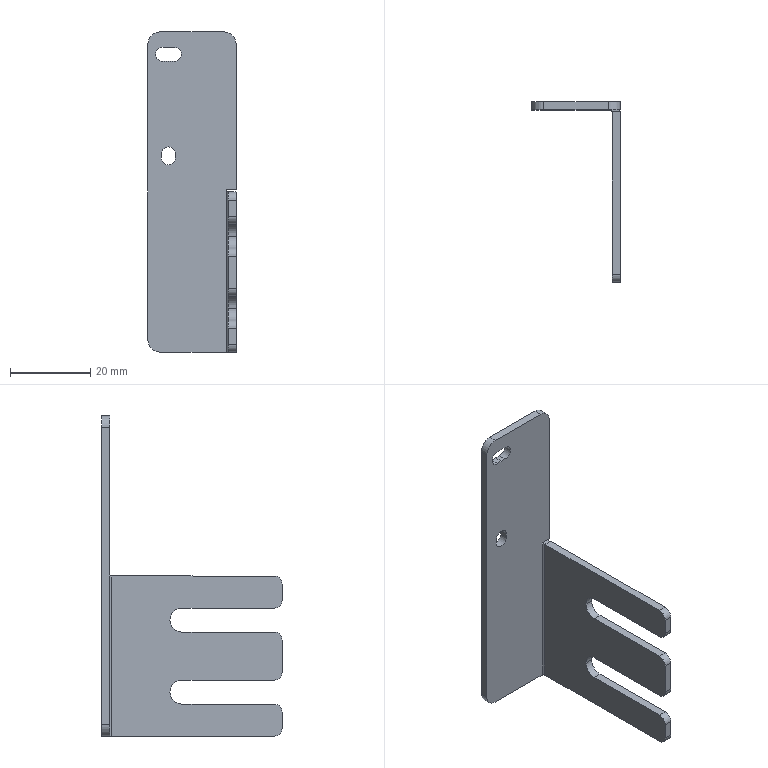Part | SolidWorks | features ICE 4, Fillet 2, ExtruThin 1, FlatPattern 1, FlattenBends 1, ProcessBends 1, SheetMetal 1 | 1 solid | 47 faces | box 22 x 45 x 80 mm | volume 6161 mm3 | cylinder 24 | plane 23 | commonest cylinder face diameters 6 x7 4 x6 3.5 x5 47.3 x2 54.3 x2 1 x1
STEP:
#1=CARTESIAN_POINT('',(-2.,-17.,29.));
#2=VERTEX_POINT('',#1);
#3=CARTESIAN_POINT('',(-2.,-20.,32.));
#4=VERTEX_POINT('',#3);
#5=CARTESIAN_POINT('',(-2.,-20.,29.));
#6=DIRECTION('',(1.,0.,0.));
#7=DIRECTION('',(0.,1.,0.));
#8=AXIS2_PLACEMENT_3D('',#5,#6,#7);
#9=CIRCLE('',#8,3.);
#10=EDGE_CURVE('',#2,#4,#9,.T.);
#11=ORIENTED_EDGE('',*,*,#10,.F.);
#12=CARTESIAN_POINT('',(0.,-17.,29.));
#13=VERTEX_POINT('',#12);
#14=CARTESIAN_POINT('',(-116.726,-17.,29.));
#15=DIRECTION('',(1.,0.,0.));
#16=VECTOR('',#15,1000.);
#17=LINE('',#14,#16);
#18=EDGE_CURVE('',#2,#13,#17,.T.);
#19=ORIENTED_EDGE('',*,*,#18,.T.);
#20=CARTESIAN_POINT('',(0.,-20.,32.));
#21=VERTEX_POINT('',#20);
#22=CARTESIAN_POINT('',(0.,-20.,29.));
#23=DIRECTION('',(1.,0.,0.));
#24=DIRECTION('',(0.,1.,0.));
#25=AXIS2_PLACEMENT_3D('',#22,#23,#24);
#26=CIRCLE('',#25,3.);
#27=EDGE_CURVE('',#13,#21,#26,.T.);
#28=ORIENTED_EDGE('',*,*,#27,.T.);
#29=CARTESIAN_POINT('',(-116.726,-20.,32.));
#30=DIRECTION('',(1.,0.,0.));
#31=VECTOR('',#30,1000.);
#32=LINE('',#29,#31);
#33=EDGE_CURVE('',#4,#21,#32,.T.);
#34=ORIENTED_EDGE('',*,*,#33,.F.);
#35=EDGE_LOOP('',(#11,#19,#28,#34));
#36=FACE_OUTER_BOUND('',#35,.T.);
#37=CARTESIAN_POINT('',(-116.726,-20.,29.));
#38=DIRECTION('',(1.,0.,0.));
#39=DIRECTION('',(0.,1.,0.));
#40=AXIS2_PLACEMENT_3D('',#37,#38,#39);
#41=CYLINDRICAL_SURFACE('',#40,3.);
#42=ADVANCED_FACE('',(#36),#41,.F.);
#43=CARTESIAN_POINT('',(-2.,-17.,11.));
#44=VERTEX_POINT('',#43);
#45=CARTESIAN_POINT('',(-2.,-20.,14.));
#46=VERTEX_POINT('',#45);
#47=CARTESIAN_POINT('',(-2.,-20.,11.));
#48=DIRECTION('',(1.,0.,0.));
#49=DIRECTION('',(0.,1.,0.));
#50=AXIS2_PLACEMENT_3D('',#47,#48,#49);
#51=CIRCLE('',#50,3.);
#52=EDGE_CURVE('',#44,#46,#51,.T.);
#53=ORIENTED_EDGE('',*,*,#52,.F.);
#54=CARTESIAN_POINT('',(0.,-17.,11.));
#55=VERTEX_POINT('',#54);
#56=CARTESIAN_POINT('',(-116.726,-17.,11.));
#57=DIRECTION('',(1.,0.,0.));
#58=VECTOR('',#57,1000.);
#59=LINE('',#56,#58);
#60=EDGE_CURVE('',#44,#55,#59,.T.);
#61=ORIENTED_EDGE('',*,*,#60,.T.);
#62=CARTESIAN_POINT('',(0.,-20.,14.));
#63=VERTEX_POINT('',#62);
#64=CARTESIAN_POINT('',(0.,-20.,11.));
#65=DIRECTION('',(1.,0.,0.));
#66=DIRECTION('',(0.,-1.,0.));
#67=AXIS2_PLACEMENT_3D('',#64,#65,#66);
#68=CIRCLE('',#67,3.);
#69=EDGE_CURVE('',#55,#63,#68,.T.);
#70=ORIENTED_EDGE('',*,*,#69,.T.);
#71=CARTESIAN_POINT('',(-116.726,-20.,14.));
#72=DIRECTION('',(1.,0.,0.));
#73=VECTOR('',#72,1000.);
#74=LINE('',#71,#73);
#75=EDGE_CURVE('',#46,#63,#74,.T.);
#76=ORIENTED_EDGE('',*,*,#75,.F.);
#77=EDGE_LOOP('',(#53,#61,#70,#76));
#78=FACE_OUTER_BOUND('',#77,.T.);
#79=CARTESIAN_POINT('',(-116.726,-20.,11.));
#80=DIRECTION('',(1.,0.,0.));
#81=DIRECTION('',(0.,1.,0.));
#82=AXIS2_PLACEMENT_3D('',#79,#80,#81);
#83=CYLINDRICAL_SURFACE('',#82,3.);
#84=ADVANCED_FACE('',(#78),#83,.F.);
#85=CARTESIAN_POINT('',(-16.893,-2.,51.25));
#86=VERTEX_POINT('',#85);
#87=CARTESIAN_POINT('',(-15.143,-2.,49.5));
#88=VERTEX_POINT('',#87);
#89=CARTESIAN_POINT('',(-16.893,-2.,49.5));
#90=DIRECTION('',(0.,1.,0.));
#91=DIRECTION('',(0.,0.,1.));
#92=AXIS2_PLACEMENT_3D('',#89,#90,#91);
#93=CIRCLE('',#92,1.75);
#94=EDGE_CURVE('',#86,#88,#93,.T.);
#95=ORIENTED_EDGE('',*,*,#94,.F.);
#96=CARTESIAN_POINT('',(-16.893,0.,51.25));
#97=VERTEX_POINT('',#96);
#98=CARTESIAN_POINT('',(-16.893,-10.,51.25));
#99=DIRECTION('',(0.,1.,0.));
#100=VECTOR('',#99,1000.);
#101=LINE('',#98,#100);
#102=EDGE_CURVE('',#86,#97,#101,.T.);
#103=ORIENTED_EDGE('',*,*,#102,.T.);
#104=CARTESIAN_POINT('',(-15.143,0.,49.5));
#105=VERTEX_POINT('',#104);
#106=CARTESIAN_POINT('',(-16.893,0.,49.5));
#107=DIRECTION('',(0.,1.,0.));
#108=DIRECTION('',(0.,0.,1.));
#109=AXIS2_PLACEMENT_3D('',#106,#107,#108);
#110=CIRCLE('',#109,1.75);
#111=EDGE_CURVE('',#97,#105,#110,.T.);
#112=ORIENTED_EDGE('',*,*,#111,.T.);
#113=CARTESIAN_POINT('',(-15.143,-10.,49.5));
#114=DIRECTION('',(0.,1.,0.));
#115=VECTOR('',#114,1000.);
#116=LINE('',#113,#115);
#117=EDGE_CURVE('',#88,#105,#116,.T.);
#118=ORIENTED_EDGE('',*,*,#117,.F.);
#119=EDGE_LOOP('',(#95,#103,#112,#118));
#120=FACE_OUTER_BOUND('',#119,.T.);
#121=CARTESIAN_POINT('',(-16.893,-10.,49.5));
#122=DIRECTION('',(0.,1.,0.));
#123=DIRECTION('',(0.,0.,1.));
#124=AXIS2_PLACEMENT_3D('',#121,#122,#123);
#125=CYLINDRICAL_SURFACE('',#124,1.75);
#126=ADVANCED_FACE('',(#120),#125,.F.);
#127=CARTESIAN_POINT('',(-16.893,-2.,72.65));
#128=VERTEX_POINT('',#127);
#129=CARTESIAN_POINT('',(-18.289,-2.,72.609));
#130=VERTEX_POINT('',#129);
#131=CARTESIAN_POINT('',(-16.893,-2.,49.));
#132=DIRECTION('',(0.,-1.,0.));
#133=DIRECTION('',(0.,0.,1.));
#134=AXIS2_PLACEMENT_3D('',#131,#132,#133);
#135=CIRCLE('',#134,23.65);
#136=EDGE_CURVE('',#128,#130,#135,.T.);
#137=ORIENTED_EDGE('',*,*,#136,.F.);
#138=CARTESIAN_POINT('',(-16.893,0.,72.65));
#139=VERTEX_POINT('',#138);
#140=CARTESIAN_POINT('',(-16.893,-10.,72.65));
#141=DIRECTION('',(0.,1.,0.));
#142=VECTOR('',#141,1000.);
#143=LINE('',#140,#142);
#144=EDGE_CURVE('',#128,#139,#143,.T.);
#145=ORIENTED_EDGE('',*,*,#144,.T.);
#146=CARTESIAN_POINT('',(-18.289,0.,72.609));
#147=VERTEX_POINT('',#146);
#148=CARTESIAN_POINT('',(-16.893,0.,49.));
#149=DIRECTION('',(0.,-1.,0.));
#150=DIRECTION('',(0.,0.,1.));
#151=AXIS2_PLACEMENT_3D('',#148,#149,#150);
#152=CIRCLE('',#151,23.65);
#153=EDGE_CURVE('',#139,#147,#152,.T.);
#154=ORIENTED_EDGE('',*,*,#153,.T.);
#155=CARTESIAN_POINT('',(-18.289,-10.,72.609));
#156=DIRECTION('',(0.,1.,0.));
#157=VECTOR('',#156,1000.);
#158=LINE('',#155,#157);
#159=EDGE_CURVE('',#130,#147,#158,.T.);
#160=ORIENTED_EDGE('',*,*,#159,.F.);
#161=EDGE_LOOP('',(#137,#145,#154,#160));
#162=FACE_OUTER_BOUND('',#161,.T.);
#163=CARTESIAN_POINT('',(-16.893,-10.,49.));
#164=DIRECTION('',(0.,1.,0.));
#165=DIRECTION('',(0.,0.,1.));
#166=AXIS2_PLACEMENT_3D('',#163,#164,#165);
#167=CYLINDRICAL_SURFACE('',#166,23.65);
#168=ADVANCED_FACE('',(#162),#167,.T.);
#169=CARTESIAN_POINT('',(-16.893,-2.,76.15));
#170=VERTEX_POINT('',#169);
#171=CARTESIAN_POINT('',(-15.289,-2.,76.103));
#172=VERTEX_POINT('',#171);
#173=CARTESIAN_POINT('',(-16.893,-2.,49.));
#174=DIRECTION('',(0.,1.,0.));
#175=DIRECTION('',(0.,0.,1.));
#176=AXIS2_PLACEMENT_3D('',#173,#174,#175);
#177=CIRCLE('',#176,27.15);
#178=EDGE_CURVE('',#170,#172,#177,.T.);
#179=ORIENTED_EDGE('',*,*,#178,.F.);
#180=CARTESIAN_POINT('',(-16.893,0.,76.15));
#181=VERTEX_POINT('',#180);
#182=CARTESIAN_POINT('',(-16.893,-10.,76.15));
#183=DIRECTION('',(0.,1.,0.));
#184=VECTOR('',#183,1000.);
#185=LINE('',#182,#184);
#186=EDGE_CURVE('',#170,#181,#185,.T.);
#187=ORIENTED_EDGE('',*,*,#186,.T.);
#188=CARTESIAN_POINT('',(-15.289,0.,76.103));
#189=VERTEX_POINT('',#188);
#190=CARTESIAN_POINT('',(-16.893,0.,49.));
#191=DIRECTION('',(0.,1.,0.));
#192=DIRECTION('',(0.,0.,1.));
#193=AXIS2_PLACEMENT_3D('',#190,#191,#192);
#194=CIRCLE('',#193,27.15);
#195=EDGE_CURVE('',#181,#189,#194,.T.);
#196=ORIENTED_EDGE('',*,*,#195,.T.);
#197=CARTESIAN_POINT('',(-15.289,-10.,76.103));
#198=DIRECTION('',(0.,1.,0.));
#199=VECTOR('',#198,1000.);
#200=LINE('',#197,#199);
#201=EDGE_CURVE('',#172,#189,#200,.T.);
#202=ORIENTED_EDGE('',*,*,#201,.F.);
#203=EDGE_LOOP('',(#179,#187,#196,#202));
#204=FACE_OUTER_BOUND('',#203,.T.);
#205=CARTESIAN_POINT('',(-16.893,-10.,49.));
#206=DIRECTION('',(0.,1.,0.));
#207=DIRECTION('',(0.,0.,1.));
#208=AXIS2_PLACEMENT_3D('',#205,#206,#207);
#209=CYLINDRICAL_SURFACE('',#208,27.15);
#210=ADVANCED_FACE('',(#204),#209,.F.);
#211=ORIENTED_EDGE('',*,*,#186,.F.);
#212=CARTESIAN_POINT('',(-18.496,-2.,76.103));
#213=VERTEX_POINT('',#212);
#214=CARTESIAN_POINT('',(-16.893,-2.,49.));
#215=DIRECTION('',(0.,1.,0.));
#216=DIRECTION('',(0.,0.,1.));
#217=AXIS2_PLACEMENT_3D('',#214,#215,#216);
#218=CIRCLE('',#217,27.15);
#219=EDGE_CURVE('',#213,#170,#218,.T.);
#220=ORIENTED_EDGE('',*,*,#219,.F.);
#221=CARTESIAN_POINT('',(-18.496,0.,76.103));
#222=VERTEX_POINT('',#221);
#223=CARTESIAN_POINT('',(-18.496,-10.,76.103));
#224=DIRECTION('',(0.,1.,0.));
#225=VECTOR('',#224,1000.);
#226=LINE('',#223,#225);
#227=EDGE_CURVE('',#213,#222,#226,.T.);
#228=ORIENTED_EDGE('',*,*,#227,.T.);
#229=CARTESIAN_POINT('',(-16.893,0.,49.));
#230=DIRECTION('',(0.,1.,0.));
#231=DIRECTION('',(0.,0.,1.));
#232=AXIS2_PLACEMENT_3D('',#229,#230,#231);
#233=CIRCLE('',#232,27.15);
#234=EDGE_CURVE('',#222,#181,#233,.T.);
#235=ORIENTED_EDGE('',*,*,#234,.T.);
#236=EDGE_LOOP('',(#211,#220,#228,#235));
#237=FACE_OUTER_BOUND('',#236,.T.);
#238=CARTESIAN_POINT('',(-16.893,-10.,49.));
#239=DIRECTION('',(0.,1.,0.));
#240=DIRECTION('',(0.,0.,1.));
#241=AXIS2_PLACEMENT_3D('',#238,#239,#240);
#242=CYLINDRICAL_SURFACE('',#241,27.15);
#243=ADVANCED_FACE('',(#237),#242,.F.);
#244=ORIENTED_EDGE('',*,*,#201,.T.);
#245=CARTESIAN_POINT('',(-15.496,0.,72.609));
#246=VERTEX_POINT('',#245);
#247=CARTESIAN_POINT('',(-15.393,0.,74.356));
#248=DIRECTION('',(0.,1.,0.));
#249=DIRECTION('',(0.,0.,1.));
#250=AXIS2_PLACEMENT_3D('',#247,#248,#249);
#251=CIRCLE('',#250,1.75);
#252=EDGE_CURVE('',#189,#246,#251,.T.);
#253=ORIENTED_EDGE('',*,*,#252,.T.);
#254=CARTESIAN_POINT('',(-15.496,-2.,72.609));
#255=VERTEX_POINT('',#254);
#256=CARTESIAN_POINT('',(-15.496,-10.,72.609));
#257=DIRECTION('',(0.,1.,0.));
#258=VECTOR('',#257,1000.);
#259=LINE('',#256,#258);
#260=EDGE_CURVE('',#255,#246,#259,.T.);
#261=ORIENTED_EDGE('',*,*,#260,.F.);
#262=CARTESIAN_POINT('',(-15.393,-2.,74.356));
#263=DIRECTION('',(0.,1.,0.));
#264=DIRECTION('',(0.,0.,1.));
#265=AXIS2_PLACEMENT_3D('',#262,#263,#264);
#266=CIRCLE('',#265,1.75);
#267=EDGE_CURVE('',#172,#255,#266,.T.);
#268=ORIENTED_EDGE('',*,*,#267,.F.);
#269=EDGE_LOOP('',(#244,#253,#261,#268));
#270=FACE_OUTER_BOUND('',#269,.T.);
#271=CARTESIAN_POINT('',(-15.393,-10.,74.356));
#272=DIRECTION('',(0.,1.,0.));
#273=DIRECTION('',(0.,0.,1.));
#274=AXIS2_PLACEMENT_3D('',#271,#272,#273);
#275=CYLINDRICAL_SURFACE('',#274,1.75);
#276=ADVANCED_FACE('',(#270),#275,.F.);
#277=ORIENTED_EDGE('',*,*,#144,.F.);
#278=CARTESIAN_POINT('',(-16.893,-2.,49.));
#279=DIRECTION('',(0.,-1.,0.));
#280=DIRECTION('',(0.,0.,1.));
#281=AXIS2_PLACEMENT_3D('',#278,#279,#280);
#282=CIRCLE('',#281,23.65);
#283=EDGE_CURVE('',#255,#128,#282,.T.);
#284=ORIENTED_EDGE('',*,*,#283,.F.);
#285=ORIENTED_EDGE('',*,*,#260,.T.);
#286=CARTESIAN_POINT('',(-16.893,0.,49.));
#287=DIRECTION('',(0.,-1.,0.));
#288=DIRECTION('',(0.,0.,1.));
#289=AXIS2_PLACEMENT_3D('',#286,#287,#288);
#290=CIRCLE('',#289,23.65);
#291=EDGE_CURVE('',#246,#139,#290,.T.);
#292=ORIENTED_EDGE('',*,*,#291,.T.);
#293=EDGE_LOOP('',(#277,#284,#285,#292));
#294=FACE_OUTER_BOUND('',#293,.T.);
#295=CARTESIAN_POINT('',(-16.893,-10.,49.));
#296=DIRECTION('',(0.,1.,0.));
#297=DIRECTION('',(0.,0.,1.));
#298=AXIS2_PLACEMENT_3D('',#295,#296,#297);
#299=CYLINDRICAL_SURFACE('',#298,23.65);
#300=ADVANCED_FACE('',(#294),#299,.T.);
#301=ORIENTED_EDGE('',*,*,#159,.T.);
#302=CARTESIAN_POINT('',(-18.393,0.,74.356));
#303=DIRECTION('',(0.,1.,0.));
#304=DIRECTION('',(0.,0.,1.));
#305=AXIS2_PLACEMENT_3D('',#302,#303,#304);
#306=CIRCLE('',#305,1.75);
#307=EDGE_CURVE('',#147,#222,#306,.T.);
#308=ORIENTED_EDGE('',*,*,#307,.T.);
#309=ORIENTED_EDGE('',*,*,#227,.F.);
#310=CARTESIAN_POINT('',(-18.393,-2.,74.356));
#311=DIRECTION('',(0.,1.,0.));
#312=DIRECTION('',(0.,0.,1.));
#313=AXIS2_PLACEMENT_3D('',#310,#311,#312);
#314=CIRCLE('',#313,1.75);
#315=EDGE_CURVE('',#130,#213,#314,.T.);
#316=ORIENTED_EDGE('',*,*,#315,.F.);
#317=EDGE_LOOP('',(#301,#308,#309,#316));
#318=FACE_OUTER_BOUND('',#317,.T.);
#319=CARTESIAN_POINT('',(-18.393,-10.,74.356));
#320=DIRECTION('',(0.,1.,0.));
#321=DIRECTION('',(0.,0.,1.));
#322=AXIS2_PLACEMENT_3D('',#319,#320,#321);
#323=CYLINDRICAL_SURFACE('',#322,1.75);
#324=ADVANCED_FACE('',(#318),#323,.F.);
#325=ORIENTED_EDGE('',*,*,#117,.T.);
#326=CARTESIAN_POINT('',(-15.143,0.,48.5));
#327=VERTEX_POINT('',#326);
#328=CARTESIAN_POINT('',(-15.143,0.,49.5));
#329=DIRECTION('',(0.,0.,-1.));
#330=VECTOR('',#329,1000.);
#331=LINE('',#328,#330);
#332=EDGE_CURVE('',#105,#327,#331,.T.);
#333=ORIENTED_EDGE('',*,*,#332,.T.);
#334=CARTESIAN_POINT('',(-15.143,-2.,48.5));
#335=VERTEX_POINT('',#334);
#336=CARTESIAN_POINT('',(-15.143,-10.,48.5));
#337=DIRECTION('',(0.,1.,0.));
#338=VECTOR('',#337,1000.);
#339=LINE('',#336,#338);
#340=EDGE_CURVE('',#335,#327,#339,.T.);
#341=ORIENTED_EDGE('',*,*,#340,.F.);
#342=CARTESIAN_POINT('',(-15.143,-2.,80.));
#343=DIRECTION('',(0.,0.,-1.));
#344=VECTOR('',#343,1000.);
#345=LINE('',#342,#344);
#346=EDGE_CURVE('',#88,#335,#345,.T.);
#347=ORIENTED_EDGE('',*,*,#346,.F.);
#348=EDGE_LOOP('',(#325,#333,#341,#347));
#349=FACE_OUTER_BOUND('',#348,.T.);
#350=CARTESIAN_POINT('',(-15.143,-10.,49.5));
#351=DIRECTION('',(1.,0.,0.));
#352=DIRECTION('',(0.,0.,-1.));
#353=AXIS2_PLACEMENT_3D('',#350,#351,#352);
#354=PLANE('',#353);
#355=ADVANCED_FACE('',(#349),#354,.F.);
#356=ORIENTED_EDGE('',*,*,#340,.T.);
#357=CARTESIAN_POINT('',(-18.643,0.,48.5));
#358=VERTEX_POINT('',#357);
#359=CARTESIAN_POINT('',(-16.893,0.,48.5));
#360=DIRECTION('',(0.,1.,0.));
#361=DIRECTION('',(0.,0.,1.));
#362=AXIS2_PLACEMENT_3D('',#359,#360,#361);
#363=CIRCLE('',#362,1.75);
#364=EDGE_CURVE('',#327,#358,#363,.T.);
#365=ORIENTED_EDGE('',*,*,#364,.T.);
#366=CARTESIAN_POINT('',(-18.643,-2.,48.5));
#367=VERTEX_POINT('',#366);
#368=CARTESIAN_POINT('',(-18.643,-10.,48.5));
#369=DIRECTION('',(0.,1.,0.));
#370=VECTOR('',#369,1000.);
#371=LINE('',#368,#370);
#372=EDGE_CURVE('',#367,#358,#371,.T.);
#373=ORIENTED_EDGE('',*,*,#372,.F.);
#374=CARTESIAN_POINT('',(-16.893,-2.,48.5));
#375=DIRECTION('',(0.,1.,0.));
#376=DIRECTION('',(0.,0.,1.));
#377=AXIS2_PLACEMENT_3D('',#374,#375,#376);
#378=CIRCLE('',#377,1.75);
#379=EDGE_CURVE('',#335,#367,#378,.T.);
#380=ORIENTED_EDGE('',*,*,#379,.F.);
#381=EDGE_LOOP('',(#356,#365,#373,#380));
#382=FACE_OUTER_BOUND('',#381,.T.);
#383=CARTESIAN_POINT('',(-16.893,-10.,48.5));
#384=DIRECTION('',(0.,1.,0.));
#385=DIRECTION('',(0.,0.,1.));
#386=AXIS2_PLACEMENT_3D('',#383,#384,#385);
#387=CYLINDRICAL_SURFACE('',#386,1.75);
#388=ADVANCED_FACE('',(#382),#387,.F.);
#389=ORIENTED_EDGE('',*,*,#372,.T.);
#390=CARTESIAN_POINT('',(-18.643,0.,49.5));
#391=VERTEX_POINT('',#390);
#392=CARTESIAN_POINT('',(-18.643,0.,49.5));
#393=DIRECTION('',(0.,0.,1.));
#394=VECTOR('',#393,1000.);
#395=LINE('',#392,#394);
#396=EDGE_CURVE('',#358,#391,#395,.T.);
#397=ORIENTED_EDGE('',*,*,#396,.T.);
#398=CARTESIAN_POINT('',(-18.643,-2.,49.5));
#399=VERTEX_POINT('',#398);
#400=CARTESIAN_POINT('',(-18.643,-10.,49.5));
#401=DIRECTION('',(0.,1.,0.));
#402=VECTOR('',#401,1000.);
#403=LINE('',#400,#402);
#404=EDGE_CURVE('',#399,#391,#403,.T.);
#405=ORIENTED_EDGE('',*,*,#404,.F.);
#406=CARTESIAN_POINT('',(-18.643,-2.,80.));
#407=DIRECTION('',(0.,0.,1.));
#408=VECTOR('',#407,1000.);
#409=LINE('',#406,#408);
#410=EDGE_CURVE('',#367,#399,#409,.T.);
#411=ORIENTED_EDGE('',*,*,#410,.F.);
#412=EDGE_LOOP('',(#389,#397,#405,#411));
#413=FACE_OUTER_BOUND('',#412,.T.);
#414=CARTESIAN_POINT('',(-18.643,-10.,49.5));
#415=DIRECTION('',(-1.,0.,0.));
#416=DIRECTION('',(0.,0.,1.));
#417=AXIS2_PLACEMENT_3D('',#414,#415,#416);
#418=PLANE('',#417);
#419=ADVANCED_FACE('',(#413),#418,.F.);
#420=ORIENTED_EDGE('',*,*,#102,.F.);
#421=CARTESIAN_POINT('',(-16.893,-2.,49.5));
#422=DIRECTION('',(0.,1.,0.));
#423=DIRECTION('',(0.,0.,1.));
#424=AXIS2_PLACEMENT_3D('',#421,#422,#423);
#425=CIRCLE('',#424,1.75);
#426=EDGE_CURVE('',#399,#86,#425,.T.);
#427=ORIENTED_EDGE('',*,*,#426,.F.);
#428=ORIENTED_EDGE('',*,*,#404,.T.);
#429=CARTESIAN_POINT('',(-16.893,0.,49.5));
#430=DIRECTION('',(0.,1.,0.));
#431=DIRECTION('',(0.,0.,1.));
#432=AXIS2_PLACEMENT_3D('',#429,#430,#431);
#433=CIRCLE('',#432,1.75);
#434=EDGE_CURVE('',#391,#97,#433,.T.);
#435=ORIENTED_EDGE('',*,*,#434,.T.);
#436=EDGE_LOOP('',(#420,#427,#428,#435));
#437=FACE_OUTER_BOUND('',#436,.T.);
#438=CARTESIAN_POINT('',(-16.893,-10.,49.5));
#439=DIRECTION('',(0.,1.,0.));
#440=DIRECTION('',(0.,0.,1.));
#441=AXIS2_PLACEMENT_3D('',#438,#439,#440);
#442=CYLINDRICAL_SURFACE('',#441,1.75);
#443=ADVANCED_FACE('',(#437),#442,.F.);
#444=CARTESIAN_POINT('',(0.,-2.,40.5));
#445=VERTEX_POINT('',#444);
#446=CARTESIAN_POINT('',(0.,0.,40.5));
#447=VERTEX_POINT('',#446);
#448=CARTESIAN_POINT('',(0.,-165.94,40.5));
#449=DIRECTION('',(0.,1.,0.));
#450=VECTOR('',#449,1000.);
#451=LINE('',#448,#450);
#452=EDGE_CURVE('',#445,#447,#451,.T.);
#453=ORIENTED_EDGE('',*,*,#452,.T.);
#454=CARTESIAN_POINT('',(0.,0.,77.));
#455=VERTEX_POINT('',#454);
#456=CARTESIAN_POINT('',(0.,0.,80.));
#457=DIRECTION('',(0.,0.,-1.));
#458=VECTOR('',#457,1000.);
#459=LINE('',#456,#458);
#460=EDGE_CURVE('',#455,#447,#459,.T.);
#461=ORIENTED_EDGE('',*,*,#460,.F.);
#462=CARTESIAN_POINT('',(0.,-2.,77.));
#463=VERTEX_POINT('',#462);
#464=CARTESIAN_POINT('',(0.,-165.94,77.));
#465=DIRECTION('',(0.,1.,0.));
#466=VECTOR('',#465,1000.);
#467=LINE('',#464,#466);
#468=EDGE_CURVE('',#463,#455,#467,.T.);
#469=ORIENTED_EDGE('',*,*,#468,.F.);
#470=CARTESIAN_POINT('',(0.,-2.,80.));
#471=DIRECTION('',(0.,0.,-1.));
#472=VECTOR('',#471,1000.);
#473=LINE('',#470,#472);
#474=EDGE_CURVE('',#463,#445,#473,.T.);
#475=ORIENTED_EDGE('',*,*,#474,.T.);
#476=EDGE_LOOP('',(#453,#461,#469,#475));
#477=FACE_OUTER_BOUND('',#476,.T.);
#478=CARTESIAN_POINT('',(0.,-165.94,80.));
#479=DIRECTION('',(1.,0.,0.));
#480=DIRECTION('',(0.,1.,0.));
#481=AXIS2_PLACEMENT_3D('',#478,#479,#480);
#482=PLANE('',#481);
#483=ADVANCED_FACE('',(#477),#482,.T.);
#484=CARTESIAN_POINT('',(-3.,0.,80.));
#485=VERTEX_POINT('',#484);
#486=CARTESIAN_POINT('',(-3.,0.,77.));
#487=DIRECTION('',(0.,1.,0.));
#488=DIRECTION('',(0.,0.,1.));
#489=AXIS2_PLACEMENT_3D('',#486,#487,#488);
#490=CIRCLE('',#489,3.);
#491=EDGE_CURVE('',#485,#455,#490,.T.);
#492=ORIENTED_EDGE('',*,*,#491,.F.);
#493=CARTESIAN_POINT('',(-3.,-2.,80.));
#494=VERTEX_POINT('',#493);
#495=CARTESIAN_POINT('',(-3.,-165.94,80.));
#496=DIRECTION('',(0.,1.,0.));
#497=VECTOR('',#496,1000.);
#498=LINE('',#495,#497);
#499=EDGE_CURVE('',#494,#485,#498,.T.);
#500=ORIENTED_EDGE('',*,*,#499,.F.);
#501=CARTESIAN_POINT('',(-3.,-2.,77.));
#502=DIRECTION('',(0.,-1.,0.));
#503=DIRECTION('',(0.,0.,1.));
#504=AXIS2_PLACEMENT_3D('',#501,#502,#503);
#505=CIRCLE('',#504,3.);
#506=EDGE_CURVE('',#463,#494,#505,.T.);
#507=ORIENTED_EDGE('',*,*,#506,.F.);
#508=ORIENTED_EDGE('',*,*,#468,.T.);
#509=EDGE_LOOP('',(#492,#500,#507,#508));
#510=FACE_OUTER_BOUND('',#509,.T.);
#511=CARTESIAN_POINT('',(-3.,-165.94,77.));
#512=DIRECTION('',(0.,1.,0.));
#513=DIRECTION('',(-1.,0.,0.));
#514=AXIS2_PLACEMENT_3D('',#511,#512,#513);
#515=CYLINDRICAL_SURFACE('',#514,3.);
#516=ADVANCED_FACE('',(#510),#515,.T.);
#517=ORIENTED_EDGE('',*,*,#499,.T.);
#518=CARTESIAN_POINT('',(-19.,0.,80.));
#519=VERTEX_POINT('',#518);
#520=CARTESIAN_POINT('',(-22.,0.,80.));
#521=DIRECTION('',(1.,0.,0.));
#522=VECTOR('',#521,1000.);
#523=LINE('',#520,#522);
#524=EDGE_CURVE('',#519,#485,#523,.T.);
#525=ORIENTED_EDGE('',*,*,#524,.F.);
#526=CARTESIAN_POINT('',(-19.,-2.,80.));
#527=VERTEX_POINT('',#526);
#528=CARTESIAN_POINT('',(-19.,-165.94,80.));
#529=DIRECTION('',(0.,1.,0.));
#530=VECTOR('',#529,1000.);
#531=LINE('',#528,#530);
#532=EDGE_CURVE('',#527,#519,#531,.T.);
#533=ORIENTED_EDGE('',*,*,#532,.F.);
#534=CARTESIAN_POINT('',(-22.,-2.,80.));
#535=DIRECTION('',(1.,0.,0.));
#536=VECTOR('',#535,1000.);
#537=LINE('',#534,#536);
#538=EDGE_CURVE('',#527,#494,#537,.T.);
#539=ORIENTED_EDGE('',*,*,#538,.T.);
#540=EDGE_LOOP('',(#517,#525,#533,#539));
#541=FACE_OUTER_BOUND('',#540,.T.);
#542=CARTESIAN_POINT('',(-22.,-165.94,80.));
#543=DIRECTION('',(0.,0.,1.));
#544=DIRECTION('',(0.,1.,0.));
#545=AXIS2_PLACEMENT_3D('',#542,#543,#544);
#546=PLANE('',#545);
#547=ADVANCED_FACE('',(#541),#546,.T.);
#548=CARTESIAN_POINT('',(-22.,0.,77.));
#549=VERTEX_POINT('',#548);
#550=CARTESIAN_POINT('',(-19.,0.,77.));
#551=DIRECTION('',(0.,1.,0.));
#552=DIRECTION('',(0.,0.,1.));
#553=AXIS2_PLACEMENT_3D('',#550,#551,#552);
#554=CIRCLE('',#553,3.);
#555=EDGE_CURVE('',#549,#519,#554,.T.);
#556=ORIENTED_EDGE('',*,*,#555,.F.);
#557=CARTESIAN_POINT('',(-22.,-2.,77.));
#558=VERTEX_POINT('',#557);
#559=CARTESIAN_POINT('',(-22.,-165.94,77.));
#560=DIRECTION('',(0.,1.,0.));
#561=VECTOR('',#560,1000.);
#562=LINE('',#559,#561);
#563=EDGE_CURVE('',#558,#549,#562,.T.);
#564=ORIENTED_EDGE('',*,*,#563,.F.);
#565=CARTESIAN_POINT('',(-19.,-2.,77.));
#566=DIRECTION('',(0.,-1.,0.));
#567=DIRECTION('',(0.,0.,1.));
#568=AXIS2_PLACEMENT_3D('',#565,#566,#567);
#569=CIRCLE('',#568,3.);
#570=EDGE_CURVE('',#527,#558,#569,.T.);
#571=ORIENTED_EDGE('',*,*,#570,.F.);
#572=ORIENTED_EDGE('',*,*,#532,.T.);
#573=EDGE_LOOP('',(#556,#564,#571,#572));
#574=FACE_OUTER_BOUND('',#573,.T.);
#575=CARTESIAN_POINT('',(-19.,-165.94,77.));
#576=DIRECTION('',(0.,1.,0.));
#577=DIRECTION('',(-1.,0.,0.));
#578=AXIS2_PLACEMENT_3D('',#575,#576,#577);
#579=CYLINDRICAL_SURFACE('',#578,3.);
#580=ADVANCED_FACE('',(#574),#579,.T.);
#581=CARTESIAN_POINT('',(-22.,0.,3.));
#582=VERTEX_POINT('',#581);
#583=CARTESIAN_POINT('',(-22.,0.,80.));
#584=DIRECTION('',(0.,0.,-1.));
#585=VECTOR('',#584,1000.);
#586=LINE('',#583,#585);
#587=EDGE_CURVE('',#549,#582,#586,.T.);
#588=ORIENTED_EDGE('',*,*,#587,.T.);
#589=CARTESIAN_POINT('',(-22.,-2.,3.));
#590=VERTEX_POINT('',#589);
#591=CARTESIAN_POINT('',(-22.,-165.94,3.));
#592=DIRECTION('',(0.,1.,0.));
#593=VECTOR('',#592,1000.);
#594=LINE('',#591,#593);
#595=EDGE_CURVE('',#590,#582,#594,.T.);
#596=ORIENTED_EDGE('',*,*,#595,.F.);
#597=CARTESIAN_POINT('',(-22.,-2.,80.));
#598=DIRECTION('',(0.,0.,-1.));
#599=VECTOR('',#598,1000.);
#600=LINE('',#597,#599);
#601=EDGE_CURVE('',#558,#590,#600,.T.);
#602=ORIENTED_EDGE('',*,*,#601,.F.);
#603=ORIENTED_EDGE('',*,*,#563,.T.);
#604=EDGE_LOOP('',(#588,#596,#602,#603));
#605=FACE_OUTER_BOUND('',#604,.T.);
#606=CARTESIAN_POINT('',(-22.,-165.94,80.));
#607=DIRECTION('',(1.,0.,0.));
#608=DIRECTION('',(0.,1.,0.));
#609=AXIS2_PLACEMENT_3D('',#606,#607,#608);
#610=PLANE('',#609);
#611=ADVANCED_FACE('',(#605),#610,.F.);
#612=CARTESIAN_POINT('',(-19.,0.,0.));
#613=VERTEX_POINT('',#612);
#614=CARTESIAN_POINT('',(-19.,0.,3.));
#615=DIRECTION('',(0.,1.,0.));
#616=DIRECTION('',(0.,0.,1.));
#617=AXIS2_PLACEMENT_3D('',#614,#615,#616);
#618=CIRCLE('',#617,3.);
#619=EDGE_CURVE('',#613,#582,#618,.T.);
#620=ORIENTED_EDGE('',*,*,#619,.F.);
#621=CARTESIAN_POINT('',(-19.,-2.,0.));
#622=VERTEX_POINT('',#621);
#623=CARTESIAN_POINT('',(-19.,-165.94,0.));
#624=DIRECTION('',(0.,1.,0.));
#625=VECTOR('',#624,1000.);
#626=LINE('',#623,#625);
#627=EDGE_CURVE('',#622,#613,#626,.T.);
#628=ORIENTED_EDGE('',*,*,#627,.F.);
#629=CARTESIAN_POINT('',(-19.,-2.,3.));
#630=DIRECTION('',(0.,-1.,0.));
#631=DIRECTION('',(0.,0.,1.));
#632=AXIS2_PLACEMENT_3D('',#629,#630,#631);
#633=CIRCLE('',#632,3.);
#634=EDGE_CURVE('',#590,#622,#633,.T.);
#635=ORIENTED_EDGE('',*,*,#634,.F.);
#636=ORIENTED_EDGE('',*,*,#595,.T.);
#637=EDGE_LOOP('',(#620,#628,#635,#636));
#638=FACE_OUTER_BOUND('',#637,.T.);
#639=CARTESIAN_POINT('',(-19.,-165.94,3.));
#640=DIRECTION('',(0.,1.,0.));
#641=DIRECTION('',(-1.,0.,0.));
#642=AXIS2_PLACEMENT_3D('',#639,#640,#641);
#643=CYLINDRICAL_SURFACE('',#642,3.);
#644=ADVANCED_FACE('',(#638),#643,.T.);
#645=CARTESIAN_POINT('',(-2.5,0.,40.5));
#646=VERTEX_POINT('',#645);
#647=CARTESIAN_POINT('',(-22.,0.,40.5));
#648=DIRECTION('',(1.,0.,0.));
#649=VECTOR('',#648,1000.);
#650=LINE('',#647,#649);
#651=EDGE_CURVE('',#646,#447,#650,.T.);
#652=ORIENTED_EDGE('',*,*,#651,.T.);
#653=ORIENTED_EDGE('',*,*,#452,.F.);
#654=CARTESIAN_POINT('',(-2.5,-2.,40.5));
#655=VERTEX_POINT('',#654);
#656=CARTESIAN_POINT('',(-2.5,-2.,40.5));
#657=DIRECTION('',(1.,0.,0.));
#658=VECTOR('',#657,1000.);
#659=LINE('',#656,#658);
#660=EDGE_CURVE('',#655,#445,#659,.T.);
#661=ORIENTED_EDGE('',*,*,#660,.F.);
#662=CARTESIAN_POINT('',(-2.5,-165.94,40.5));
#663=DIRECTION('',(0.,1.,0.));
#664=VECTOR('',#663,1000.);
#665=LINE('',#662,#664);
#666=EDGE_CURVE('',#655,#646,#665,.T.);
#667=ORIENTED_EDGE('',*,*,#666,.T.);
#668=EDGE_LOOP('',(#652,#653,#661,#667));
#669=FACE_OUTER_BOUND('',#668,.T.);
#670=CARTESIAN_POINT('',(-2.5,-165.94,40.5));
#671=DIRECTION('',(0.,0.,1.));
#672=DIRECTION('',(0.,1.,0.));
#673=AXIS2_PLACEMENT_3D('',#670,#671,#672);
#674=PLANE('',#673);
#675=ADVANCED_FACE('',(#669),#674,.F.);
#676=CARTESIAN_POINT('',(-2.5,-2.,40.));
#677=VERTEX_POINT('',#676);
#678=CARTESIAN_POINT('',(-2.5,0.,40.));
#679=VERTEX_POINT('',#678);
#680=CARTESIAN_POINT('',(-2.5,-165.94,40.));
#681=DIRECTION('',(0.,1.,0.));
#682=VECTOR('',#681,1000.);
#683=LINE('',#680,#682);
#684=EDGE_CURVE('',#677,#679,#683,.T.);
#685=ORIENTED_EDGE('',*,*,#684,.T.);
#686=CARTESIAN_POINT('',(-2.5,0.,80.));
#687=DIRECTION('',(0.,0.,-1.));
#688=VECTOR('',#687,1000.);
#689=LINE('',#686,#688);
#690=EDGE_CURVE('',#646,#679,#689,.T.);
#691=ORIENTED_EDGE('',*,*,#690,.F.);
#692=ORIENTED_EDGE('',*,*,#666,.F.);
#693=CARTESIAN_POINT('',(-2.5,-2.,40.));
#694=DIRECTION('',(0.,0.,-1.));
#695=VECTOR('',#694,1000.);
#696=LINE('',#693,#695);
#697=EDGE_CURVE('',#655,#677,#696,.T.);
#698=ORIENTED_EDGE('',*,*,#697,.T.);
#699=EDGE_LOOP('',(#685,#691,#692,#698));
#700=FACE_OUTER_BOUND('',#699,.T.);
#701=CARTESIAN_POINT('',(-2.5,-165.94,40.));
#702=DIRECTION('',(1.,0.,0.));
#703=DIRECTION('',(0.,1.,0.));
#704=AXIS2_PLACEMENT_3D('',#701,#702,#703);
#705=PLANE('',#704);
#706=ADVANCED_FACE('',(#700),#705,.T.);
#707=CARTESIAN_POINT('',(-2.5,0.,0.));
#708=VERTEX_POINT('',#707);
#709=CARTESIAN_POINT('',(-2.5,0.,40.));
#710=DIRECTION('',(0.,0.,1.));
#711=VECTOR('',#710,1000.);
#712=LINE('',#709,#711);
#713=EDGE_CURVE('',#708,#679,#712,.T.);
#714=ORIENTED_EDGE('',*,*,#713,.F.);
#715=CARTESIAN_POINT('',(-22.,0.,0.));
#716=DIRECTION('',(1.,0.,0.));
#717=VECTOR('',#716,1000.);
#718=LINE('',#715,#717);
#719=EDGE_CURVE('',#613,#708,#718,.T.);
#720=ORIENTED_EDGE('',*,*,#719,.F.);
#721=ORIENTED_EDGE('',*,*,#619,.T.);
#722=ORIENTED_EDGE('',*,*,#587,.F.);
#723=ORIENTED_EDGE('',*,*,#555,.T.);
#724=ORIENTED_EDGE('',*,*,#524,.T.);
#725=ORIENTED_EDGE('',*,*,#491,.T.);
#726=ORIENTED_EDGE('',*,*,#460,.T.);
#727=ORIENTED_EDGE('',*,*,#651,.F.);
#728=ORIENTED_EDGE('',*,*,#690,.T.);
#729=EDGE_LOOP('',(#714,#720,#721,#722,#723,#724,#725,#726,#727,#728));
#730=FACE_OUTER_BOUND('',#729,.T.);
#731=ORIENTED_EDGE('',*,*,#434,.F.);
#732=ORIENTED_EDGE('',*,*,#396,.F.);
#733=ORIENTED_EDGE('',*,*,#364,.F.);
#734=ORIENTED_EDGE('',*,*,#332,.F.);
#735=ORIENTED_EDGE('',*,*,#111,.F.);
#736=EDGE_LOOP('',(#731,#732,#733,#734,#735));
#737=FACE_BOUND('',#736,.T.);
#738=ORIENTED_EDGE('',*,*,#307,.F.);
#739=ORIENTED_EDGE('',*,*,#153,.F.);
#740=ORIENTED_EDGE('',*,*,#291,.F.);
#741=ORIENTED_EDGE('',*,*,#252,.F.);
#742=ORIENTED_EDGE('',*,*,#195,.F.);
#743=ORIENTED_EDGE('',*,*,#234,.F.);
#744=EDGE_LOOP('',(#738,#739,#740,#741,#742,#743));
#745=FACE_BOUND('',#744,.T.);
#746=CARTESIAN_POINT('',(-22.,0.,80.));
#747=DIRECTION('',(0.,1.,0.));
#748=DIRECTION('',(0.,0.,1.));
#749=AXIS2_PLACEMENT_3D('',#746,#747,#748);
#750=PLANE('',#749);
#751=ADVANCED_FACE('',(#730,#737,#745),#750,.T.);
#752=ORIENTED_EDGE('',*,*,#719,.T.);
#753=CARTESIAN_POINT('',(-2.5,-2.,0.));
#754=VERTEX_POINT('',#753);
#755=CARTESIAN_POINT('',(-2.5,-165.94,0.));
#756=DIRECTION('',(0.,1.,0.));
#757=VECTOR('',#756,1000.);
#758=LINE('',#755,#757);
#759=EDGE_CURVE('',#754,#708,#758,.T.);
#760=ORIENTED_EDGE('',*,*,#759,.F.);
#761=CARTESIAN_POINT('',(-22.,-2.,0.));
#762=DIRECTION('',(1.,0.,0.));
#763=VECTOR('',#762,1000.);
#764=LINE('',#761,#763);
#765=EDGE_CURVE('',#622,#754,#764,.T.);
#766=ORIENTED_EDGE('',*,*,#765,.F.);
#767=ORIENTED_EDGE('',*,*,#627,.T.);
#768=EDGE_LOOP('',(#752,#760,#766,#767));
#769=FACE_OUTER_BOUND('',#768,.T.);
#770=CARTESIAN_POINT('',(-22.,-165.94,0.));
#771=DIRECTION('',(0.,0.,1.));
#772=DIRECTION('',(0.,1.,0.));
#773=AXIS2_PLACEMENT_3D('',#770,#771,#772);
#774=PLANE('',#773);
#775=ADVANCED_FACE('',(#769),#774,.F.);
#776=ORIENTED_EDGE('',*,*,#765,.T.);
#777=CARTESIAN_POINT('',(-2.5,-2.,40.));
#778=DIRECTION('',(0.,0.,1.));
#779=VECTOR('',#778,1000.);
#780=LINE('',#777,#779);
#781=EDGE_CURVE('',#754,#677,#780,.T.);
#782=ORIENTED_EDGE('',*,*,#781,.T.);
#783=ORIENTED_EDGE('',*,*,#697,.F.);
#784=ORIENTED_EDGE('',*,*,#660,.T.);
#785=ORIENTED_EDGE('',*,*,#474,.F.);
#786=ORIENTED_EDGE('',*,*,#506,.T.);
#787=ORIENTED_EDGE('',*,*,#538,.F.);
#788=ORIENTED_EDGE('',*,*,#570,.T.);
#789=ORIENTED_EDGE('',*,*,#601,.T.);
#790=ORIENTED_EDGE('',*,*,#634,.T.);
#791=EDGE_LOOP('',(#776,#782,#783,#784,#785,#786,#787,#788,#789,#790));
#792=FACE_OUTER_BOUND('',#791,.T.);
#793=ORIENTED_EDGE('',*,*,#410,.T.);
#794=ORIENTED_EDGE('',*,*,#426,.T.);
#795=ORIENTED_EDGE('',*,*,#94,.T.);
#796=ORIENTED_EDGE('',*,*,#346,.T.);
#797=ORIENTED_EDGE('',*,*,#379,.T.);
#798=EDGE_LOOP('',(#793,#794,#795,#796,#797));
#799=FACE_BOUND('',#798,.T.);
#800=ORIENTED_EDGE('',*,*,#283,.T.);
#801=ORIENTED_EDGE('',*,*,#136,.T.);
#802=ORIENTED_EDGE('',*,*,#315,.T.);
#803=ORIENTED_EDGE('',*,*,#219,.T.);
#804=ORIENTED_EDGE('',*,*,#178,.T.);
#805=ORIENTED_EDGE('',*,*,#267,.T.);
#806=EDGE_LOOP('',(#800,#801,#802,#803,#804,#805));
#807=FACE_BOUND('',#806,.T.);
#808=CARTESIAN_POINT('',(-22.,-2.,80.));
#809=DIRECTION('',(0.,1.,0.));
#810=DIRECTION('',(0.,0.,1.));
#811=AXIS2_PLACEMENT_3D('',#808,#809,#810);
#812=PLANE('',#811);
#813=ADVANCED_FACE('',(#792,#799,#807),#812,.F.);
#814=CARTESIAN_POINT('',(-2.,-43.,40.));
#815=VERTEX_POINT('',#814);
#816=CARTESIAN_POINT('',(0.,-43.,40.));
#817=VERTEX_POINT('',#816);
#818=CARTESIAN_POINT('',(-116.726,-43.,40.));
#819=DIRECTION('',(1.,0.,0.));
#820=VECTOR('',#819,1000.);
#821=LINE('',#818,#820);
#822=EDGE_CURVE('',#815,#817,#821,.T.);
#823=ORIENTED_EDGE('',*,*,#822,.T.);
#824=CARTESIAN_POINT('',(0.,-2.5,40.));
#825=VERTEX_POINT('',#824);
#826=CARTESIAN_POINT('',(0.,-45.,40.));
#827=DIRECTION('',(0.,-1.,0.));
#828=VECTOR('',#827,1000.);
#829=LINE('',#826,#828);
#830=EDGE_CURVE('',#825,#817,#829,.T.);
#831=ORIENTED_EDGE('',*,*,#830,.F.);
#832=CARTESIAN_POINT('',(-2.,-2.5,40.));
#833=VERTEX_POINT('',#832);
#834=CARTESIAN_POINT('',(-116.726,-2.5,40.));
#835=DIRECTION('',(1.,0.,0.));
#836=VECTOR('',#835,1000.);
#837=LINE('',#834,#836);
#838=EDGE_CURVE('',#833,#825,#837,.T.);
#839=ORIENTED_EDGE('',*,*,#838,.F.);
#840=CARTESIAN_POINT('',(-2.,-45.,40.));
#841=DIRECTION('',(0.,-1.,0.));
#842=VECTOR('',#841,1000.);
#843=LINE('',#840,#842);
#844=EDGE_CURVE('',#833,#815,#843,.T.);
#845=ORIENTED_EDGE('',*,*,#844,.T.);
#846=EDGE_LOOP('',(#823,#831,#839,#845));
#847=FACE_OUTER_BOUND('',#846,.T.);
#848=CARTESIAN_POINT('',(-116.726,-45.,40.));
#849=DIRECTION('',(0.,0.,1.));
#850=DIRECTION('',(1.,0.,0.));
#851=AXIS2_PLACEMENT_3D('',#848,#849,#850);
#852=PLANE('',#851);
#853=ADVANCED_FACE('',(#847),#852,.T.);
#854=CARTESIAN_POINT('',(0.,-2.5,0.));
#855=VERTEX_POINT('',#854);
#856=CARTESIAN_POINT('',(0.,-43.,0.));
#857=VERTEX_POINT('',#856);
#858=CARTESIAN_POINT('',(0.,0.,0.));
#859=DIRECTION('',(0.,-1.,0.));
#860=VECTOR('',#859,1000.);
#861=LINE('',#858,#860);
#862=EDGE_CURVE('',#855,#857,#861,.T.);
#863=ORIENTED_EDGE('',*,*,#862,.T.);
#864=CARTESIAN_POINT('',(-2.,-43.,0.));
#865=VERTEX_POINT('',#864);
#866=CARTESIAN_POINT('',(-116.726,-43.,0.));
#867=DIRECTION('',(1.,0.,0.));
#868=VECTOR('',#867,1000.);
#869=LINE('',#866,#868);
#870=EDGE_CURVE('',#865,#857,#869,.T.);
#871=ORIENTED_EDGE('',*,*,#870,.F.);
#872=CARTESIAN_POINT('',(-2.,-2.5,0.));
#873=VERTEX_POINT('',#872);
#874=CARTESIAN_POINT('',(-2.,0.,0.));
#875=DIRECTION('',(0.,-1.,0.));
#876=VECTOR('',#875,1000.);
#877=LINE('',#874,#876);
#878=EDGE_CURVE('',#873,#865,#877,.T.);
#879=ORIENTED_EDGE('',*,*,#878,.F.);
#880=CARTESIAN_POINT('',(-116.726,-2.5,0.));
#881=DIRECTION('',(1.,0.,0.));
#882=VECTOR('',#881,1000.);
#883=LINE('',#880,#882);
#884=EDGE_CURVE('',#873,#855,#883,.T.);
#885=ORIENTED_EDGE('',*,*,#884,.T.);
#886=EDGE_LOOP('',(#863,#871,#879,#885));
#887=FACE_OUTER_BOUND('',#886,.T.);
#888=CARTESIAN_POINT('',(-116.726,0.,0.));
#889=DIRECTION('',(0.,0.,1.));
#890=DIRECTION('',(1.,0.,0.));
#891=AXIS2_PLACEMENT_3D('',#888,#889,#890);
#892=PLANE('',#891);
#893=ADVANCED_FACE('',(#887),#892,.F.);
#894=CARTESIAN_POINT('',(0.,-45.,2.));
#895=VERTEX_POINT('',#894);
#896=CARTESIAN_POINT('',(0.,-43.,2.));
#897=DIRECTION('',(1.,0.,0.));
#898=DIRECTION('',(0.,1.,0.));
#899=AXIS2_PLACEMENT_3D('',#896,#897,#898);
#900=CIRCLE('',#899,2.);
#901=EDGE_CURVE('',#895,#857,#900,.T.);
#902=ORIENTED_EDGE('',*,*,#901,.F.);
#903=CARTESIAN_POINT('',(-2.,-45.,2.));
#904=VERTEX_POINT('',#903);
#905=CARTESIAN_POINT('',(-116.726,-45.,2.));
#906=DIRECTION('',(1.,0.,0.));
#907=VECTOR('',#906,1000.);
#908=LINE('',#905,#907);
#909=EDGE_CURVE('',#904,#895,#908,.T.);
#910=ORIENTED_EDGE('',*,*,#909,.F.);
#911=CARTESIAN_POINT('',(-2.,-43.,2.));
#912=DIRECTION('',(-1.,0.,0.));
#913=DIRECTION('',(0.,1.,0.));
#914=AXIS2_PLACEMENT_3D('',#911,#912,#913);
#915=CIRCLE('',#914,2.);
#916=EDGE_CURVE('',#865,#904,#915,.T.);
#917=ORIENTED_EDGE('',*,*,#916,.F.);
#918=ORIENTED_EDGE('',*,*,#870,.T.);
#919=EDGE_LOOP('',(#902,#910,#917,#918));
#920=FACE_OUTER_BOUND('',#919,.T.);
#921=CARTESIAN_POINT('',(-116.726,-43.,2.));
#922=DIRECTION('',(1.,0.,0.));
#923=DIRECTION('',(0.,1.,0.));
#924=AXIS2_PLACEMENT_3D('',#921,#922,#923);
#925=CYLINDRICAL_SURFACE('',#924,2.);
#926=ADVANCED_FACE('',(#920),#925,.T.);
#927=ORIENTED_EDGE('',*,*,#909,.T.);
#928=CARTESIAN_POINT('',(0.,-45.,6.));
#929=VERTEX_POINT('',#928);
#930=CARTESIAN_POINT('',(0.,-45.,80.));
#931=DIRECTION('',(0.,0.,-1.));
#932=VECTOR('',#931,1000.);
#933=LINE('',#930,#932);
#934=EDGE_CURVE('',#929,#895,#933,.T.);
#935=ORIENTED_EDGE('',*,*,#934,.F.);
#936=CARTESIAN_POINT('',(-2.,-45.,6.));
#937=VERTEX_POINT('',#936);
#938=CARTESIAN_POINT('',(-116.726,-45.,6.));
#939=DIRECTION('',(1.,0.,0.));
#940=VECTOR('',#939,1000.);
#941=LINE('',#938,#940);
#942=EDGE_CURVE('',#937,#929,#941,.T.);
#943=ORIENTED_EDGE('',*,*,#942,.F.);
#944=CARTESIAN_POINT('',(-2.,-45.,80.));
#945=DIRECTION('',(0.,0.,-1.));
#946=VECTOR('',#945,1000.);
#947=LINE('',#944,#946);
#948=EDGE_CURVE('',#937,#904,#947,.T.);
#949=ORIENTED_EDGE('',*,*,#948,.T.);
#950=EDGE_LOOP('',(#927,#935,#943,#949));
#951=FACE_OUTER_BOUND('',#950,.T.);
#952=CARTESIAN_POINT('',(-116.726,-45.,80.));
#953=DIRECTION('',(0.,-1.,0.));
#954=DIRECTION('',(1.,0.,0.));
#955=AXIS2_PLACEMENT_3D('',#952,#953,#954);
#956=PLANE('',#955);
#957=ADVANCED_FACE('',(#951),#956,.T.);
#958=CARTESIAN_POINT('',(0.,-43.,8.));
#959=VERTEX_POINT('',#958);
#960=CARTESIAN_POINT('',(0.,-43.,6.));
#961=DIRECTION('',(1.,0.,0.));
#962=DIRECTION('',(0.,1.,0.));
#963=AXIS2_PLACEMENT_3D('',#960,#961,#962);
#964=CIRCLE('',#963,2.);
#965=EDGE_CURVE('',#959,#929,#964,.T.);
#966=ORIENTED_EDGE('',*,*,#965,.F.);
#967=CARTESIAN_POINT('',(-2.,-43.,8.));
#968=VERTEX_POINT('',#967);
#969=CARTESIAN_POINT('',(-116.726,-43.,8.));
#970=DIRECTION('',(1.,0.,0.));
#971=VECTOR('',#970,1000.);
#972=LINE('',#969,#971);
#973=EDGE_CURVE('',#968,#959,#972,.T.);
#974=ORIENTED_EDGE('',*,*,#973,.F.);
#975=CARTESIAN_POINT('',(-2.,-43.,6.));
#976=DIRECTION('',(-1.,0.,0.));
#977=DIRECTION('',(0.,1.,0.));
#978=AXIS2_PLACEMENT_3D('',#975,#976,#977);
#979=CIRCLE('',#978,2.);
#980=EDGE_CURVE('',#937,#968,#979,.T.);
#981=ORIENTED_EDGE('',*,*,#980,.F.);
#982=ORIENTED_EDGE('',*,*,#942,.T.);
#983=EDGE_LOOP('',(#966,#974,#981,#982));
#984=FACE_OUTER_BOUND('',#983,.T.);
#985=CARTESIAN_POINT('',(-116.726,-43.,6.));
#986=DIRECTION('',(1.,0.,0.));
#987=DIRECTION('',(0.,1.,0.));
#988=AXIS2_PLACEMENT_3D('',#985,#986,#987);
#989=CYLINDRICAL_SURFACE('',#988,2.);
#990=ADVANCED_FACE('',(#984),#989,.T.);
#991=CARTESIAN_POINT('',(0.,-20.,8.));
#992=VERTEX_POINT('',#991);
#993=CARTESIAN_POINT('',(0.,0.,8.));
#994=DIRECTION('',(0.,1.,0.));
#995=VECTOR('',#994,1000.);
#996=LINE('',#993,#995);
#997=EDGE_CURVE('',#959,#992,#996,.T.);
#998=ORIENTED_EDGE('',*,*,#997,.T.);
#999=CARTESIAN_POINT('',(-2.,-20.,8.));
#1000=VERTEX_POINT('',#999);
#1001=CARTESIAN_POINT('',(-116.726,-20.,8.));
#1002=DIRECTION('',(1.,0.,0.));
#1003=VECTOR('',#1002,1000.);
#1004=LINE('',#1001,#1003);
#1005=EDGE_CURVE('',#1000,#992,#1004,.T.);
#1006=ORIENTED_EDGE('',*,*,#1005,.F.);
#1007=CARTESIAN_POINT('',(-2.,0.,8.));
#1008=DIRECTION('',(0.,1.,0.));
#1009=VECTOR('',#1008,1000.);
#1010=LINE('',#1007,#1009);
#1011=EDGE_CURVE('',#968,#1000,#1010,.T.);
#1012=ORIENTED_EDGE('',*,*,#1011,.F.);
#1013=ORIENTED_EDGE('',*,*,#973,.T.);
#1014=EDGE_LOOP('',(#998,#1006,#1012,#1013));
#1015=FACE_OUTER_BOUND('',#1014,.T.);
#1016=CARTESIAN_POINT('',(-116.726,0.,8.));
#1017=DIRECTION('',(0.,0.,-1.));
#1018=DIRECTION('',(-1.,0.,0.));
#1019=AXIS2_PLACEMENT_3D('',#1016,#1017,#1018);
#1020=PLANE('',#1019);
#1021=ADVANCED_FACE('',(#1015),#1020,.F.);
#1022=ORIENTED_EDGE('',*,*,#60,.F.);
#1023=CARTESIAN_POINT('',(-2.,-20.,11.));
#1024=DIRECTION('',(1.,0.,0.));
#1025=DIRECTION('',(0.,1.,0.));
#1026=AXIS2_PLACEMENT_3D('',#1023,#1024,#1025);
#1027=CIRCLE('',#1026,3.);
#1028=EDGE_CURVE('',#1000,#44,#1027,.T.);
#1029=ORIENTED_EDGE('',*,*,#1028,.F.);
#1030=ORIENTED_EDGE('',*,*,#1005,.T.);
#1031=CARTESIAN_POINT('',(0.,-20.,11.));
#1032=DIRECTION('',(1.,0.,0.));
#1033=DIRECTION('',(0.,-1.,0.));
#1034=AXIS2_PLACEMENT_3D('',#1031,#1032,#1033);
#1035=CIRCLE('',#1034,3.);
#1036=EDGE_CURVE('',#992,#55,#1035,.T.);
#1037=ORIENTED_EDGE('',*,*,#1036,.T.);
#1038=EDGE_LOOP('',(#1022,#1029,#1030,#1037));
#1039=FACE_OUTER_BOUND('',#1038,.T.);
#1040=CARTESIAN_POINT('',(-116.726,-20.,11.));
#1041=DIRECTION('',(1.,0.,0.));
#1042=DIRECTION('',(0.,1.,0.));
#1043=AXIS2_PLACEMENT_3D('',#1040,#1041,#1042);
#1044=CYLINDRICAL_SURFACE('',#1043,3.);
#1045=ADVANCED_FACE('',(#1039),#1044,.F.);
#1046=CARTESIAN_POINT('',(0.,-43.,14.));
#1047=VERTEX_POINT('',#1046);
#1048=CARTESIAN_POINT('',(0.,-70.,14.));
#1049=DIRECTION('',(0.,-1.,0.));
#1050=VECTOR('',#1049,1000.);
#1051=LINE('',#1048,#1050);
#1052=EDGE_CURVE('',#63,#1047,#1051,.T.);
#1053=ORIENTED_EDGE('',*,*,#1052,.T.);
#1054=CARTESIAN_POINT('',(-2.,-43.,14.));
#1055=VERTEX_POINT('',#1054);
#1056=CARTESIAN_POINT('',(-116.726,-43.,14.));
#1057=DIRECTION('',(1.,0.,0.));
#1058=VECTOR('',#1057,1000.);
#1059=LINE('',#1056,#1058);
#1060=EDGE_CURVE('',#1055,#1047,#1059,.T.);
#1061=ORIENTED_EDGE('',*,*,#1060,.F.);
#1062=CARTESIAN_POINT('',(-2.,0.,14.));
#1063=DIRECTION('',(0.,-1.,0.));
#1064=VECTOR('',#1063,1000.);
#1065=LINE('',#1062,#1064);
#1066=EDGE_CURVE('',#46,#1055,#1065,.T.);
#1067=ORIENTED_EDGE('',*,*,#1066,.F.);
#1068=ORIENTED_EDGE('',*,*,#75,.T.);
#1069=EDGE_LOOP('',(#1053,#1061,#1067,#1068));
#1070=FACE_OUTER_BOUND('',#1069,.T.);
#1071=CARTESIAN_POINT('',(-116.726,0.,14.));
#1072=DIRECTION('',(0.,0.,1.));
#1073=DIRECTION('',(1.,0.,0.));
#1074=AXIS2_PLACEMENT_3D('',#1071,#1072,#1073);
#1075=PLANE('',#1074);
#1076=ADVANCED_FACE('',(#1070),#1075,.F.);
#1077=CARTESIAN_POINT('',(0.,-45.,16.));
#1078=VERTEX_POINT('',#1077);
#1079=CARTESIAN_POINT('',(0.,-43.,16.));
#1080=DIRECTION('',(1.,0.,0.));
#1081=DIRECTION('',(0.,1.,0.));
#1082=AXIS2_PLACEMENT_3D('',#1079,#1080,#1081);
#1083=CIRCLE('',#1082,2.);
#1084=EDGE_CURVE('',#1078,#1047,#1083,.T.);
#1085=ORIENTED_EDGE('',*,*,#1084,.F.);
#1086=CARTESIAN_POINT('',(-2.,-45.,16.));
#1087=VERTEX_POINT('',#1086);
#1088=CARTESIAN_POINT('',(-116.726,-45.,16.));
#1089=DIRECTION('',(1.,0.,0.));
#1090=VECTOR('',#1089,1000.);
#1091=LINE('',#1088,#1090);
#1092=EDGE_CURVE('',#1087,#1078,#1091,.T.);
#1093=ORIENTED_EDGE('',*,*,#1092,.F.);
#1094=CARTESIAN_POINT('',(-2.,-43.,16.));
#1095=DIRECTION('',(-1.,0.,0.));
#1096=DIRECTION('',(0.,1.,0.));
#1097=AXIS2_PLACEMENT_3D('',#1094,#1095,#1096);
#1098=CIRCLE('',#1097,2.);
#1099=EDGE_CURVE('',#1055,#1087,#1098,.T.);
#1100=ORIENTED_EDGE('',*,*,#1099,.F.);
#1101=ORIENTED_EDGE('',*,*,#1060,.T.);
#1102=EDGE_LOOP('',(#1085,#1093,#1100,#1101));
#1103=FACE_OUTER_BOUND('',#1102,.T.);
#1104=CARTESIAN_POINT('',(-116.726,-43.,16.));
#1105=DIRECTION('',(1.,0.,0.));
#1106=DIRECTION('',(0.,1.,0.));
#1107=AXIS2_PLACEMENT_3D('',#1104,#1105,#1106);
#1108=CYLINDRICAL_SURFACE('',#1107,2.);
#1109=ADVANCED_FACE('',(#1103),#1108,.T.);
#1110=ORIENTED_EDGE('',*,*,#1092,.T.);
#1111=CARTESIAN_POINT('',(0.,-45.,24.));
#1112=VERTEX_POINT('',#1111);
#1113=CARTESIAN_POINT('',(0.,-45.,80.));
#1114=DIRECTION('',(0.,0.,-1.));
#1115=VECTOR('',#1114,1000.);
#1116=LINE('',#1113,#1115);
#1117=EDGE_CURVE('',#1112,#1078,#1116,.T.);
#1118=ORIENTED_EDGE('',*,*,#1117,.F.);
#1119=CARTESIAN_POINT('',(-2.,-45.,24.));
#1120=VERTEX_POINT('',#1119);
#1121=CARTESIAN_POINT('',(-116.726,-45.,24.));
#1122=DIRECTION('',(1.,0.,0.));
#1123=VECTOR('',#1122,1000.);
#1124=LINE('',#1121,#1123);
#1125=EDGE_CURVE('',#1120,#1112,#1124,.T.);
#1126=ORIENTED_EDGE('',*,*,#1125,.F.);
#1127=CARTESIAN_POINT('',(-2.,-45.,80.));
#1128=DIRECTION('',(0.,0.,-1.));
#1129=VECTOR('',#1128,1000.);
#1130=LINE('',#1127,#1129);
#1131=EDGE_CURVE('',#1120,#1087,#1130,.T.);
#1132=ORIENTED_EDGE('',*,*,#1131,.T.);
#1133=EDGE_LOOP('',(#1110,#1118,#1126,#1132));
#1134=FACE_OUTER_BOUND('',#1133,.T.);
#1135=CARTESIAN_POINT('',(-116.726,-45.,80.));
#1136=DIRECTION('',(0.,-1.,0.));
#1137=DIRECTION('',(1.,0.,0.));
#1138=AXIS2_PLACEMENT_3D('',#1135,#1136,#1137);
#1139=PLANE('',#1138);
#1140=ADVANCED_FACE('',(#1134),#1139,.T.);
#1141=CARTESIAN_POINT('',(0.,-43.,26.));
#1142=VERTEX_POINT('',#1141);
#1143=CARTESIAN_POINT('',(0.,-43.,24.));
#1144=DIRECTION('',(1.,0.,0.));
#1145=DIRECTION('',(0.,1.,0.));
#1146=AXIS2_PLACEMENT_3D('',#1143,#1144,#1145);
#1147=CIRCLE('',#1146,2.);
#1148=EDGE_CURVE('',#1142,#1112,#1147,.T.);
#1149=ORIENTED_EDGE('',*,*,#1148,.F.);
#1150=CARTESIAN_POINT('',(-2.,-43.,26.));
#1151=VERTEX_POINT('',#1150);
#1152=CARTESIAN_POINT('',(-116.726,-43.,26.));
#1153=DIRECTION('',(1.,0.,0.));
#1154=VECTOR('',#1153,1000.);
#1155=LINE('',#1152,#1154);
#1156=EDGE_CURVE('',#1151,#1142,#1155,.T.);
#1157=ORIENTED_EDGE('',*,*,#1156,.F.);
#1158=CARTESIAN_POINT('',(-2.,-43.,24.));
#1159=DIRECTION('',(-1.,0.,0.));
#1160=DIRECTION('',(0.,1.,0.));
#1161=AXIS2_PLACEMENT_3D('',#1158,#1159,#1160);
#1162=CIRCLE('',#1161,2.);
#1163=EDGE_CURVE('',#1120,#1151,#1162,.T.);
#1164=ORIENTED_EDGE('',*,*,#1163,.F.);
#1165=ORIENTED_EDGE('',*,*,#1125,.T.);
#1166=EDGE_LOOP('',(#1149,#1157,#1164,#1165));
#1167=FACE_OUTER_BOUND('',#1166,.T.);
#1168=CARTESIAN_POINT('',(-116.726,-43.,24.));
#1169=DIRECTION('',(1.,0.,0.));
#1170=DIRECTION('',(0.,1.,0.));
#1171=AXIS2_PLACEMENT_3D('',#1168,#1169,#1170);
#1172=CYLINDRICAL_SURFACE('',#1171,2.);
#1173=ADVANCED_FACE('',(#1167),#1172,.T.);
#1174=CARTESIAN_POINT('',(0.,-20.,26.));
#1175=VERTEX_POINT('',#1174);
#1176=CARTESIAN_POINT('',(0.,0.,26.));
#1177=DIRECTION('',(0.,1.,0.));
#1178=VECTOR('',#1177,1000.);
#1179=LINE('',#1176,#1178);
#1180=EDGE_CURVE('',#1142,#1175,#1179,.T.);
#1181=ORIENTED_EDGE('',*,*,#1180,.T.);
#1182=CARTESIAN_POINT('',(-2.,-20.,26.));
#1183=VERTEX_POINT('',#1182);
#1184=CARTESIAN_POINT('',(-116.726,-20.,26.));
#1185=DIRECTION('',(1.,0.,0.));
#1186=VECTOR('',#1185,1000.);
#1187=LINE('',#1184,#1186);
#1188=EDGE_CURVE('',#1183,#1175,#1187,.T.);
#1189=ORIENTED_EDGE('',*,*,#1188,.F.);
#1190=CARTESIAN_POINT('',(-2.,0.,26.));
#1191=DIRECTION('',(0.,1.,0.));
#1192=VECTOR('',#1191,1000.);
#1193=LINE('',#1190,#1192);
#1194=EDGE_CURVE('',#1151,#1183,#1193,.T.);
#1195=ORIENTED_EDGE('',*,*,#1194,.F.);
#1196=ORIENTED_EDGE('',*,*,#1156,.T.);
#1197=EDGE_LOOP('',(#1181,#1189,#1195,#1196));
#1198=FACE_OUTER_BOUND('',#1197,.T.);
#1199=CARTESIAN_POINT('',(-116.726,0.,26.));
#1200=DIRECTION('',(0.,0.,-1.));
#1201=DIRECTION('',(-1.,0.,0.));
#1202=AXIS2_PLACEMENT_3D('',#1199,#1200,#1201);
#1203=PLANE('',#1202);
#1204=ADVANCED_FACE('',(#1198),#1203,.F.);
#1205=ORIENTED_EDGE('',*,*,#18,.F.);
#1206=CARTESIAN_POINT('',(-2.,-20.,29.));
#1207=DIRECTION('',(1.,0.,0.));
#1208=DIRECTION('',(0.,1.,0.));
#1209=AXIS2_PLACEMENT_3D('',#1206,#1207,#1208);
#1210=CIRCLE('',#1209,3.);
#1211=EDGE_CURVE('',#1183,#2,#1210,.T.);
#1212=ORIENTED_EDGE('',*,*,#1211,.F.);
#1213=ORIENTED_EDGE('',*,*,#1188,.T.);
#1214=CARTESIAN_POINT('',(0.,-20.,29.));
#1215=DIRECTION('',(1.,0.,0.));
#1216=DIRECTION('',(0.,1.,0.));
#1217=AXIS2_PLACEMENT_3D('',#1214,#1215,#1216);
#1218=CIRCLE('',#1217,3.);
#1219=EDGE_CURVE('',#1175,#13,#1218,.T.);
#1220=ORIENTED_EDGE('',*,*,#1219,.T.);
#1221=EDGE_LOOP('',(#1205,#1212,#1213,#1220));
#1222=FACE_OUTER_BOUND('',#1221,.T.);
#1223=CARTESIAN_POINT('',(-116.726,-20.,29.));
#1224=DIRECTION('',(1.,0.,0.));
#1225=DIRECTION('',(0.,1.,0.));
#1226=AXIS2_PLACEMENT_3D('',#1223,#1224,#1225);
#1227=CYLINDRICAL_SURFACE('',#1226,3.);
#1228=ADVANCED_FACE('',(#1222),#1227,.F.);
#1229=CARTESIAN_POINT('',(0.,-43.,32.));
#1230=VERTEX_POINT('',#1229);
#1231=CARTESIAN_POINT('',(0.,-70.,32.));
#1232=DIRECTION('',(0.,-1.,0.));
#1233=VECTOR('',#1232,1000.);
#1234=LINE('',#1231,#1233);
#1235=EDGE_CURVE('',#21,#1230,#1234,.T.);
#1236=ORIENTED_EDGE('',*,*,#1235,.T.);
#1237=CARTESIAN_POINT('',(-2.,-43.,32.));
#1238=VERTEX_POINT('',#1237);
#1239=CARTESIAN_POINT('',(-116.726,-43.,32.));
#1240=DIRECTION('',(1.,0.,0.));
#1241=VECTOR('',#1240,1000.);
#1242=LINE('',#1239,#1241);
#1243=EDGE_CURVE('',#1238,#1230,#1242,.T.);
#1244=ORIENTED_EDGE('',*,*,#1243,.F.);
#1245=CARTESIAN_POINT('',(-2.,0.,32.));
#1246=DIRECTION('',(0.,-1.,0.));
#1247=VECTOR('',#1246,1000.);
#1248=LINE('',#1245,#1247);
#1249=EDGE_CURVE('',#4,#1238,#1248,.T.);
#1250=ORIENTED_EDGE('',*,*,#1249,.F.);
#1251=ORIENTED_EDGE('',*,*,#33,.T.);
#1252=EDGE_LOOP('',(#1236,#1244,#1250,#1251));
#1253=FACE_OUTER_BOUND('',#1252,.T.);
#1254=CARTESIAN_POINT('',(-116.726,0.,32.));
#1255=DIRECTION('',(0.,0.,1.));
#1256=DIRECTION('',(0.,-1.,0.));
#1257=AXIS2_PLACEMENT_3D('',#1254,#1255,#1256);
#1258=PLANE('',#1257);
#1259=ADVANCED_FACE('',(#1253),#1258,.F.);
#1260=CARTESIAN_POINT('',(0.,-45.,34.));
#1261=VERTEX_POINT('',#1260);
#1262=CARTESIAN_POINT('',(0.,-43.,34.));
#1263=DIRECTION('',(1.,0.,0.));
#1264=DIRECTION('',(0.,1.,0.));
#1265=AXIS2_PLACEMENT_3D('',#1262,#1263,#1264);
#1266=CIRCLE('',#1265,2.);
#1267=EDGE_CURVE('',#1261,#1230,#1266,.T.);
#1268=ORIENTED_EDGE('',*,*,#1267,.F.);
#1269=CARTESIAN_POINT('',(-2.,-45.,34.));
#1270=VERTEX_POINT('',#1269);
#1271=CARTESIAN_POINT('',(-116.726,-45.,34.));
#1272=DIRECTION('',(1.,0.,0.));
#1273=VECTOR('',#1272,1000.);
#1274=LINE('',#1271,#1273);
#1275=EDGE_CURVE('',#1270,#1261,#1274,.T.);
#1276=ORIENTED_EDGE('',*,*,#1275,.F.);
#1277=CARTESIAN_POINT('',(-2.,-43.,34.));
#1278=DIRECTION('',(-1.,0.,0.));
#1279=DIRECTION('',(0.,1.,0.));
#1280=AXIS2_PLACEMENT_3D('',#1277,#1278,#1279);
#1281=CIRCLE('',#1280,2.);
#1282=EDGE_CURVE('',#1238,#1270,#1281,.T.);
#1283=ORIENTED_EDGE('',*,*,#1282,.F.);
#1284=ORIENTED_EDGE('',*,*,#1243,.T.);
#1285=EDGE_LOOP('',(#1268,#1276,#1283,#1284));
#1286=FACE_OUTER_BOUND('',#1285,.T.);
#1287=CARTESIAN_POINT('',(-116.726,-43.,34.));
#1288=DIRECTION('',(1.,0.,0.));
#1289=DIRECTION('',(0.,1.,0.));
#1290=AXIS2_PLACEMENT_3D('',#1287,#1288,#1289);
#1291=CYLINDRICAL_SURFACE('',#1290,2.);
#1292=ADVANCED_FACE('',(#1286),#1291,.T.);
#1293=ORIENTED_EDGE('',*,*,#1275,.T.);
#1294=CARTESIAN_POINT('',(0.,-45.,38.));
#1295=VERTEX_POINT('',#1294);
#1296=CARTESIAN_POINT('',(0.,-45.,80.));
#1297=DIRECTION('',(0.,0.,-1.));
#1298=VECTOR('',#1297,1000.);
#1299=LINE('',#1296,#1298);
#1300=EDGE_CURVE('',#1295,#1261,#1299,.T.);
#1301=ORIENTED_EDGE('',*,*,#1300,.F.);
#1302=CARTESIAN_POINT('',(-2.,-45.,38.));
#1303=VERTEX_POINT('',#1302);
#1304=CARTESIAN_POINT('',(-116.726,-45.,38.));
#1305=DIRECTION('',(1.,0.,0.));
#1306=VECTOR('',#1305,1000.);
#1307=LINE('',#1304,#1306);
#1308=EDGE_CURVE('',#1303,#1295,#1307,.T.);
#1309=ORIENTED_EDGE('',*,*,#1308,.F.);
#1310=CARTESIAN_POINT('',(-2.,-45.,80.));
#1311=DIRECTION('',(0.,0.,-1.));
#1312=VECTOR('',#1311,1000.);
#1313=LINE('',#1310,#1312);
#1314=EDGE_CURVE('',#1303,#1270,#1313,.T.);
#1315=ORIENTED_EDGE('',*,*,#1314,.T.);
#1316=EDGE_LOOP('',(#1293,#1301,#1309,#1315));
#1317=FACE_OUTER_BOUND('',#1316,.T.);
#1318=CARTESIAN_POINT('',(-116.726,-45.,80.));
#1319=DIRECTION('',(0.,-1.,0.));
#1320=DIRECTION('',(1.,0.,0.));
#1321=AXIS2_PLACEMENT_3D('',#1318,#1319,#1320);
#1322=PLANE('',#1321);
#1323=ADVANCED_FACE('',(#1317),#1322,.T.);
#1324=CARTESIAN_POINT('',(0.,-43.,38.));
#1325=DIRECTION('',(1.,0.,0.));
#1326=DIRECTION('',(0.,1.,0.));
#1327=AXIS2_PLACEMENT_3D('',#1324,#1325,#1326);
#1328=CIRCLE('',#1327,2.);
#1329=EDGE_CURVE('',#817,#1295,#1328,.T.);
#1330=ORIENTED_EDGE('',*,*,#1329,.F.);
#1331=ORIENTED_EDGE('',*,*,#822,.F.);
#1332=CARTESIAN_POINT('',(-2.,-43.,38.));
#1333=DIRECTION('',(-1.,0.,0.));
#1334=DIRECTION('',(0.,1.,0.));
#1335=AXIS2_PLACEMENT_3D('',#1332,#1333,#1334);
#1336=CIRCLE('',#1335,2.);
#1337=EDGE_CURVE('',#1303,#815,#1336,.T.);
#1338=ORIENTED_EDGE('',*,*,#1337,.F.);
#1339=ORIENTED_EDGE('',*,*,#1308,.T.);
#1340=EDGE_LOOP('',(#1330,#1331,#1338,#1339));
#1341=FACE_OUTER_BOUND('',#1340,.T.);
#1342=CARTESIAN_POINT('',(-116.726,-43.,38.));
#1343=DIRECTION('',(1.,0.,0.));
#1344=DIRECTION('',(0.,1.,0.));
#1345=AXIS2_PLACEMENT_3D('',#1342,#1343,#1344);
#1346=CYLINDRICAL_SURFACE('',#1345,2.);
#1347=ADVANCED_FACE('',(#1341),#1346,.T.);
#1348=CARTESIAN_POINT('',(-2.,-2.5,40.));
#1349=DIRECTION('',(0.,0.,1.));
#1350=VECTOR('',#1349,1000.);
#1351=LINE('',#1348,#1350);
#1352=EDGE_CURVE('',#873,#833,#1351,.T.);
#1353=ORIENTED_EDGE('',*,*,#1352,.F.);
#1354=ORIENTED_EDGE('',*,*,#878,.T.);
#1355=ORIENTED_EDGE('',*,*,#916,.T.);
#1356=ORIENTED_EDGE('',*,*,#948,.F.);
#1357=ORIENTED_EDGE('',*,*,#980,.T.);
#1358=ORIENTED_EDGE('',*,*,#1011,.T.);
#1359=ORIENTED_EDGE('',*,*,#1028,.T.);
#1360=ORIENTED_EDGE('',*,*,#52,.T.);
#1361=ORIENTED_EDGE('',*,*,#1066,.T.);
#1362=ORIENTED_EDGE('',*,*,#1099,.T.);
#1363=ORIENTED_EDGE('',*,*,#1131,.F.);
#1364=ORIENTED_EDGE('',*,*,#1163,.T.);
#1365=ORIENTED_EDGE('',*,*,#1194,.T.);
#1366=ORIENTED_EDGE('',*,*,#1211,.T.);
#1367=ORIENTED_EDGE('',*,*,#10,.T.);
#1368=ORIENTED_EDGE('',*,*,#1249,.T.);
#1369=ORIENTED_EDGE('',*,*,#1282,.T.);
#1370=ORIENTED_EDGE('',*,*,#1314,.F.);
#1371=ORIENTED_EDGE('',*,*,#1337,.T.);
#1372=ORIENTED_EDGE('',*,*,#844,.F.);
#1373=EDGE_LOOP('',(#1353,#1354,#1355,#1356,#1357,#1358,#1359,#1360,#1361,#1362,#1363,#1364,#1365,#1366,#1367,#1368,#1369,#1370,#1371,#1372));
#1374=FACE_OUTER_BOUND('',#1373,.T.);
#1375=CARTESIAN_POINT('',(-2.,0.,80.));
#1376=DIRECTION('',(1.,0.,0.));
#1377=DIRECTION('',(0.,1.,0.));
#1378=AXIS2_PLACEMENT_3D('',#1375,#1376,#1377);
#1379=PLANE('',#1378);
#1380=ADVANCED_FACE('',(#1374),#1379,.F.);
#1381=ORIENTED_EDGE('',*,*,#862,.F.);
#1382=CARTESIAN_POINT('',(0.,-2.5,40.));
#1383=DIRECTION('',(0.,0.,1.));
#1384=VECTOR('',#1383,1000.);
#1385=LINE('',#1382,#1384);
#1386=EDGE_CURVE('',#855,#825,#1385,.T.);
#1387=ORIENTED_EDGE('',*,*,#1386,.T.);
#1388=ORIENTED_EDGE('',*,*,#830,.T.);
#1389=ORIENTED_EDGE('',*,*,#1329,.T.);
#1390=ORIENTED_EDGE('',*,*,#1300,.T.);
#1391=ORIENTED_EDGE('',*,*,#1267,.T.);
#1392=ORIENTED_EDGE('',*,*,#1235,.F.);
#1393=ORIENTED_EDGE('',*,*,#27,.F.);
#1394=ORIENTED_EDGE('',*,*,#1219,.F.);
#1395=ORIENTED_EDGE('',*,*,#1180,.F.);
#1396=ORIENTED_EDGE('',*,*,#1148,.T.);
#1397=ORIENTED_EDGE('',*,*,#1117,.T.);
#1398=ORIENTED_EDGE('',*,*,#1084,.T.);
#1399=ORIENTED_EDGE('',*,*,#1052,.F.);
#1400=ORIENTED_EDGE('',*,*,#69,.F.);
#1401=ORIENTED_EDGE('',*,*,#1036,.F.);
#1402=ORIENTED_EDGE('',*,*,#997,.F.);
#1403=ORIENTED_EDGE('',*,*,#965,.T.);
#1404=ORIENTED_EDGE('',*,*,#934,.T.);
#1405=ORIENTED_EDGE('',*,*,#901,.T.);
#1406=EDGE_LOOP('',(#1381,#1387,#1388,#1389,#1390,#1391,#1392,#1393,#1394,#1395,#1396,#1397,#1398,#1399,#1400,#1401,#1402,#1403,#1404,#1405));
#1407=FACE_OUTER_BOUND('',#1406,.T.);
#1408=CARTESIAN_POINT('',(0.,0.,80.));
#1409=DIRECTION('',(1.,0.,0.));
#1410=DIRECTION('',(0.,1.,0.));
#1411=AXIS2_PLACEMENT_3D('',#1408,#1409,#1410);
#1412=PLANE('',#1411);
#1413=ADVANCED_FACE('',(#1407),#1412,.T.);
#1414=ORIENTED_EDGE('',*,*,#684,.F.);
#1415=CARTESIAN_POINT('',(-2.5,-2.5,40.));
#1416=DIRECTION('',(0.,0.,-1.));
#1417=DIRECTION('',(-1.,0.,0.));
#1418=AXIS2_PLACEMENT_3D('',#1415,#1416,#1417);
#1419=CIRCLE('',#1418,0.5);
#1420=EDGE_CURVE('',#677,#833,#1419,.T.);
#1421=ORIENTED_EDGE('',*,*,#1420,.T.);
#1422=ORIENTED_EDGE('',*,*,#838,.T.);
#1423=CARTESIAN_POINT('',(-2.5,-2.5,40.));
#1424=DIRECTION('',(0.,0.,-1.));
#1425=DIRECTION('',(-1.,0.,0.));
#1426=AXIS2_PLACEMENT_3D('',#1423,#1424,#1425);
#1427=CIRCLE('',#1426,2.5);
#1428=EDGE_CURVE('',#679,#825,#1427,.T.);
#1429=ORIENTED_EDGE('',*,*,#1428,.F.);
#1430=EDGE_LOOP('',(#1414,#1421,#1422,#1429));
#1431=FACE_OUTER_BOUND('',#1430,.T.);
#1432=CARTESIAN_POINT('',(-2.5,-2.5,40.));
#1433=DIRECTION('',(0.,0.,1.));
#1434=DIRECTION('',(1.,0.,0.));
#1435=AXIS2_PLACEMENT_3D('',#1432,#1433,#1434);
#1436=PLANE('',#1435);
#1437=ADVANCED_FACE('',(#1431),#1436,.T.);
#1438=CARTESIAN_POINT('',(-2.5,-2.5,0.));
#1439=DIRECTION('',(0.,0.,1.));
#1440=DIRECTION('',(-1.,0.,0.));
#1441=AXIS2_PLACEMENT_3D('',#1438,#1439,#1440);
#1442=CIRCLE('',#1441,0.5);
#1443=EDGE_CURVE('',#873,#754,#1442,.T.);
#1444=ORIENTED_EDGE('',*,*,#1443,.T.);
#1445=ORIENTED_EDGE('',*,*,#759,.T.);
#1446=CARTESIAN_POINT('',(-2.5,-2.5,0.));
#1447=DIRECTION('',(0.,0.,1.));
#1448=DIRECTION('',(-1.,0.,0.));
#1449=AXIS2_PLACEMENT_3D('',#1446,#1447,#1448);
#1450=CIRCLE('',#1449,2.5);
#1451=EDGE_CURVE('',#855,#708,#1450,.T.);
#1452=ORIENTED_EDGE('',*,*,#1451,.F.);
#1453=ORIENTED_EDGE('',*,*,#884,.F.);
#1454=EDGE_LOOP('',(#1444,#1445,#1452,#1453));
#1455=FACE_OUTER_BOUND('',#1454,.T.);
#1456=CARTESIAN_POINT('',(-2.5,-2.5,0.));
#1457=DIRECTION('',(0.,0.,-1.));
#1458=DIRECTION('',(-1.,0.,0.));
#1459=AXIS2_PLACEMENT_3D('',#1456,#1457,#1458);
#1460=PLANE('',#1459);
#1461=ADVANCED_FACE('',(#1455),#1460,.T.);
#1462=ORIENTED_EDGE('',*,*,#1386,.F.);
#1463=ORIENTED_EDGE('',*,*,#1451,.T.);
#1464=ORIENTED_EDGE('',*,*,#713,.T.);
#1465=ORIENTED_EDGE('',*,*,#1428,.T.);
#1466=EDGE_LOOP('',(#1462,#1463,#1464,#1465));
#1467=FACE_OUTER_BOUND('',#1466,.T.);
#1468=CARTESIAN_POINT('',(-2.5,-2.5,142.202));
#1469=DIRECTION('',(0.,0.,-1.));
#1470=DIRECTION('',(-1.,0.,0.));
#1471=AXIS2_PLACEMENT_3D('',#1468,#1469,#1470);
#1472=CYLINDRICAL_SURFACE('',#1471,2.5);
#1473=ADVANCED_FACE('',(#1467),#1472,.T.);
#1474=ORIENTED_EDGE('',*,*,#1352,.T.);
#1475=ORIENTED_EDGE('',*,*,#1420,.F.);
#1476=ORIENTED_EDGE('',*,*,#781,.F.);
#1477=ORIENTED_EDGE('',*,*,#1443,.F.);
#1478=EDGE_LOOP('',(#1474,#1475,#1476,#1477));
#1479=FACE_OUTER_BOUND('',#1478,.T.);
#1480=CARTESIAN_POINT('',(-2.5,-2.5,142.202));
#1481=DIRECTION('',(0.,0.,-1.));
#1482=DIRECTION('',(-1.,0.,0.));
#1483=AXIS2_PLACEMENT_3D('',#1480,#1481,#1482);
#1484=CYLINDRICAL_SURFACE('',#1483,0.5);
#1485=ADVANCED_FACE('',(#1479),#1484,.F.);
#1486=CLOSED_SHELL('',(#42,#84,#126,#168,#210,#243,#276,#300,#324,#355,#388,#419,#443,#483,#516,#547,#580,#611,#644,#675,#706,#751,#775,#813,#853,#893,#926,#957,#990,#1021,#1045,#1076,#1109,#1140,#1173,#1204,#1228,#1259,#1292,#1323,#1347,#1380,#1413,#1437,#1461,#1473,#1485));
#1487=MANIFOLD_SOLID_BREP('',#1486);
#1488=CARTESIAN_POINT('',(0.,0.,0.));
#1489=DIRECTION('',(0.,0.,1.));
#1490=DIRECTION('',(1.,0.,0.));
#1491=AXIS2_PLACEMENT_3D('',#1488,#1489,#1490);
#1492=(LENGTH_UNIT()NAMED_UNIT(*)SI_UNIT(.MILLI.,.METRE.));
#1493=UNCERTAINTY_MEASURE_WITH_UNIT(LENGTH_MEASURE(0.00001),#1492,'','');
#1494=(NAMED_UNIT(*)PLANE_ANGLE_UNIT()SI_UNIT($,.RADIAN.));
#1495=(NAMED_UNIT(*)SI_UNIT($,.STERADIAN.)SOLID_ANGLE_UNIT());
#1496=(GEOMETRIC_REPRESENTATION_CONTEXT(3)GLOBAL_UNCERTAINTY_ASSIGNED_CONTEXT((#1493))GLOBAL_UNIT_ASSIGNED_CONTEXT((#1492,#1494,#1495))REPRESENTATION_CONTEXT('',''));
#1497=ADVANCED_BREP_SHAPE_REPRESENTATION('',(#1487,#1491),#1496);